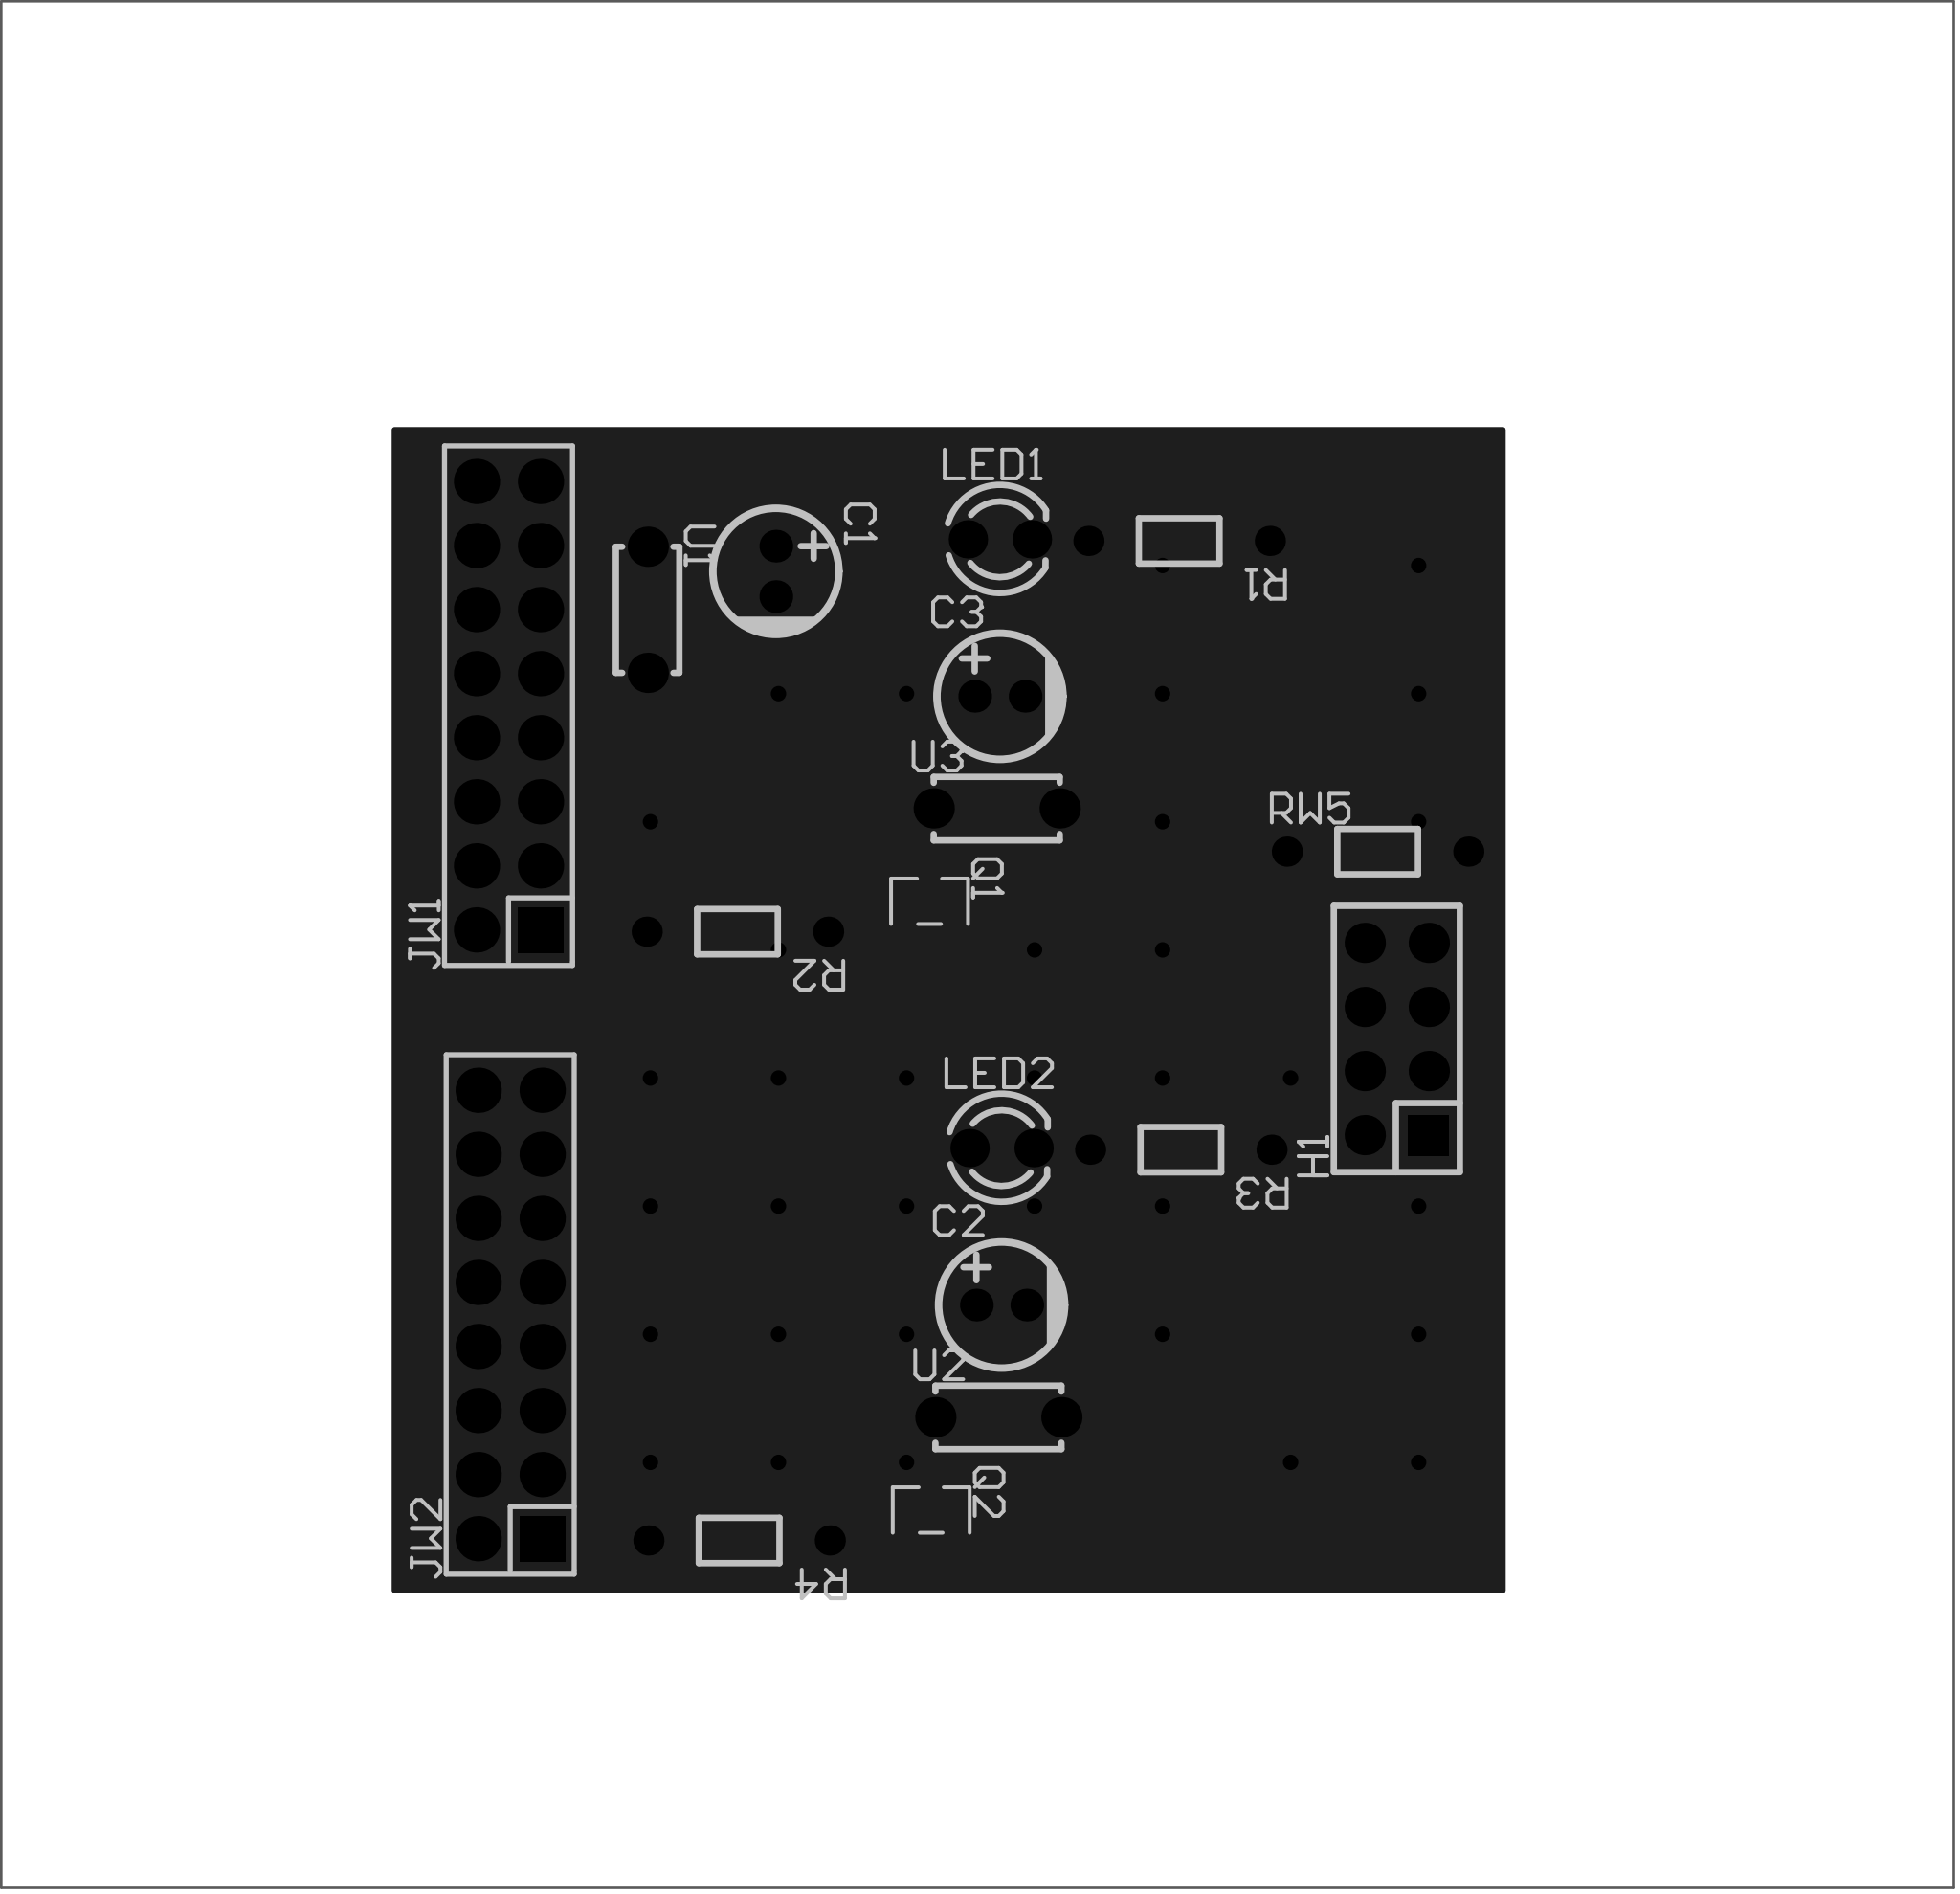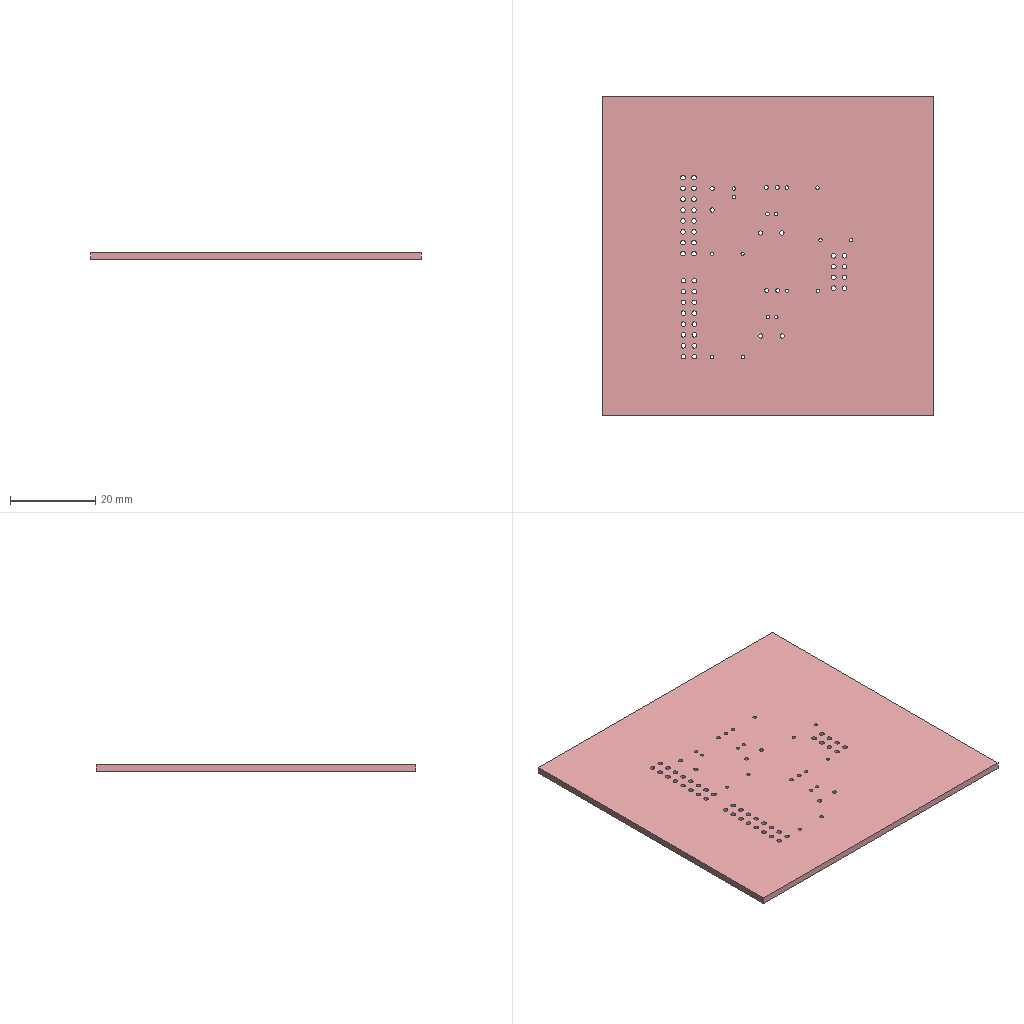Circuit board layout | Altium Designer | box 77.5 x 74.8 x 1.6 mm
Layer stack:
# Altium Designer layer stack of  (unit mm; dielectric type: 0 none, 1 core, 2 prepreg, 3 surface material)
index,name,kind,layer,copper_thickness_mm,dielectric_type,dielectric_thickness_mm,dielectric_material,dielectric_constant
0,Top Paste Mask Layer,other,,,,,,
1,Top Silkscreen Layer,other,,,,,,
2,Top Solder Mask Layer,dielectric,,,3,0.01,,3.3
3,Top Layer,copper,Top Layer,0.035,,,,
4,Dielectric1,dielectric,,,3,1.51,FR4,4.5
5,Bottom Layer,copper,Bottom Layer,0.035,,,,
6,Bottom Solder Mask Layer,dielectric,,,3,0.01,,3.3
7,Bottom Silkscreen Layer,other,,,,,,
8,Bottom Paste Mask Layer,other,,,,,,
# drill layer pairs: low layer,high layer
drill_pair,Top Layer,Bottom Layer
Part placement:
Designator,Comment,Layer,Footprint,Center-X(mm),Center-Y(mm),Rotation
C1,10uF,TopLayer,CAP-TH_BD5.0-P2.00-D0.8-FD-10UF50VC110GL,100.584,122.047,270
C2,10uF,TopLayer,CAP-TH_BD5.0-P2.00-D0.8-FD-10UF50VC110GL,109.54,92.956,0
C3,10uF,TopLayer,CAP-TH_BD5.0-P2.00-D0.8-FD-10UF50VC110GL,109.474,117.094,0
H1,,TopLayer,HDR-TH_8P-P2.54-V-F-R2-C4-S2.54-1,125.222,103.505,90
JW1,,TopLayer,HDR-TH_16P-P2.54-V-F-R2-C8-S2.54-1,89.977,116.721,90
JW2,,TopLayer,HDR-TH_16P-P2.54-V-F-R2-C8-S2.54-1,90.043,92.583,90
LED1,,TopLayer,LED_TH-3mm,109.474,123.317,0
LED2,,TopLayer,LED_TH-3mm,109.54,99.179,0
Q1,2SC2412KT146Q,TopLayer,SOT-346_L2.9-W1.6-P1.90-LS2.8-TR-CW-1,106.68,108.966,270
Q2,2SC2412KT146Q,TopLayer,SOT-346_L2.9-W1.6-P1.90-LS2.8-TR-CW-1,106.746,84.828,270
R1,100Ω,TopLayer,Res_1/8W,116.586,123.254,180
R2,100Ω,TopLayer,Res_1/8W,99.06,107.76,180
R3,100Ω,TopLayer,Res_1/8W,116.653,99.116,180
R4,100Ω,TopLayer,Res_1/8W,99.126,83.622,180
RW5,4.7kΩ,TopLayer,Res_1/8W,124.46,110.934,0
U1,100nF,TopLayer,CAP-TH_L5.0-W2.5-P5.00-D1.0,95.504,120.523,270
U2,100nF,TopLayer,CAP-TH_L5.0-W2.5-P5.00-D1.0,109.413,88.511,0
U3,100nF,TopLayer,CAP-TH_L5.0-W2.5-P5.00-D1.0,109.347,112.649,0
Pad and via stacks:
# Altium Designer via and pad stacks of  (unit mm). Each distinct definition once, with the count of objects using it.
# via: kind,start_layer,end_layer,hole_mm,diameter_mm,mode(0 simple;1 top-mid-bottom;2 full stack),diameter_per_layer,count,example_net
# pad: kind,layer,hole_mm,hole_type(0 round;1 square;2 slot),plating,top_size,top_shape(1 round;2 rect;3 octagon;9 rounded rect),mid_size,bottom_size,mode,footprint,size_per_layer,count,example
pad,Multi-Layer,0.8,0,plated,1.3x1.3,1,1.3x1.3,1.3x1.3,0,CAP-TH_BD5.0-P2.00-D0.8-FD-10UF50VC110GL,,6,C1.2
pad,Multi-Layer,1.1,0,plated,1.6x1.6,2,1.6x1.6,1.6x1.6,0,HDR-TH_8P-P2.54-V-F-R2-C4-S2.54-1,,1,H1.1
pad,Multi-Layer,1.1,0,plated,1.6x1.6,1,1.6x1.6,1.6x1.6,0,HDR-TH_8P-P2.54-V-F-R2-C4-S2.54-1,,7,H1.2
pad,Multi-Layer,1.1,0,plated,1.8x1.8,1,1.8x1.8,1.8x1.8,0,HDR-TH_16P-P2.54-V-F-R2-C8-S2.54-1,,30,JW1.16
pad,Multi-Layer,1.1,0,plated,1.8x1.8,2,1.8x1.8,1.8x1.8,0,HDR-TH_16P-P2.54-V-F-R2-C8-S2.54-1,,2,JW1.1
pad,Multi-Layer,0.9144,0,plated,1.524x1.524,1,1.524x1.524,1.524x1.524,0,LED_TH-3mm,,4,LED1.1
pad,Multi-Layer,0.8001,0,plated,1.199x1.199,1,1.199x1.199,1.199x1.199,0,Res_1/8W,,10,R1.1
pad,Multi-Layer,1,0,plated,1.6x1.6,1,1.6x1.6,1.6x1.6,0,CAP-TH_L5.0-W2.5-P5.00-D1.0,,6,U1.1
pad,Top Layer,0,0,plated,1.045x0.532,2,1.045x0.532,1.045x0.532,0,SOT-346_L2.9-W1.6-P1.90-LS2.8-TR-CW-1,,6,Q1.3
via,Top Layer,Bottom Layer,0.3048,0.61,0,,34,GND
Copper pours:
name,layer,net,type(0 solid;1 hatched;2 none)
Top Layer-GND,Top Layer,GND,0
Bottom Layer-GND,Bottom Layer,GND,0
Design rules, without the lines most boards share:
# Altium Designer design rules of  (exported by Altium Designer, unit mm)
# columns: name | kind | enabled | priority | scope1 | scope2 | descriptor | typed fields (field=value)
creepage | 65 | enabled | 1 | All | All | Creepage Distance Constraint =(0mil) (All),(All) |